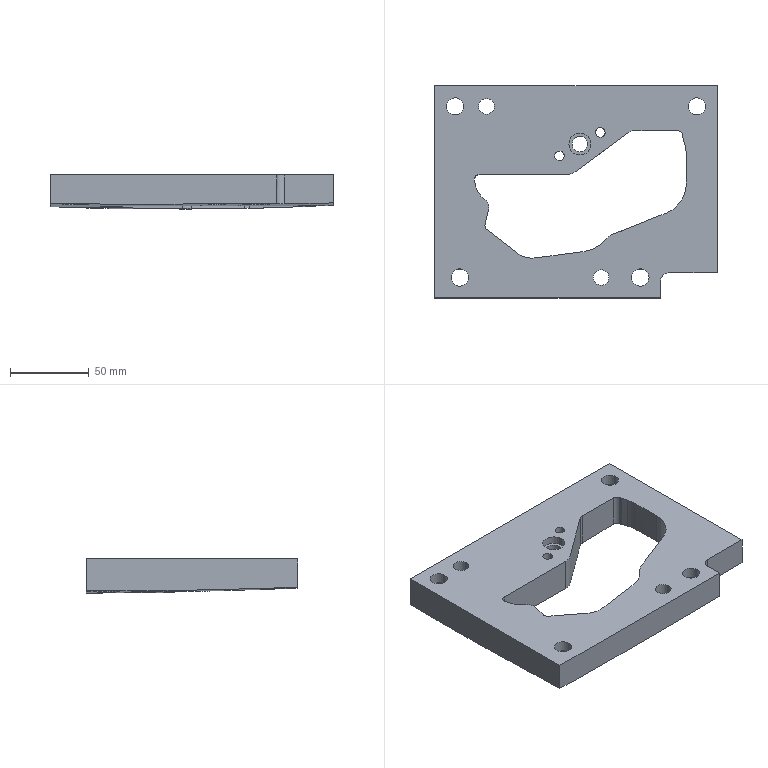Part | STEP file | 423_id1202_x_t | 1 solid | 70 faces | box 180 x 135 x 21.726 mm | volume 320962 mm3 | spline 24 | plane 23 | cylinder 23 | commonest cylinder face diameters 11 x7 10 x4 17 x4 4 x2 6 x2 6.1 x2